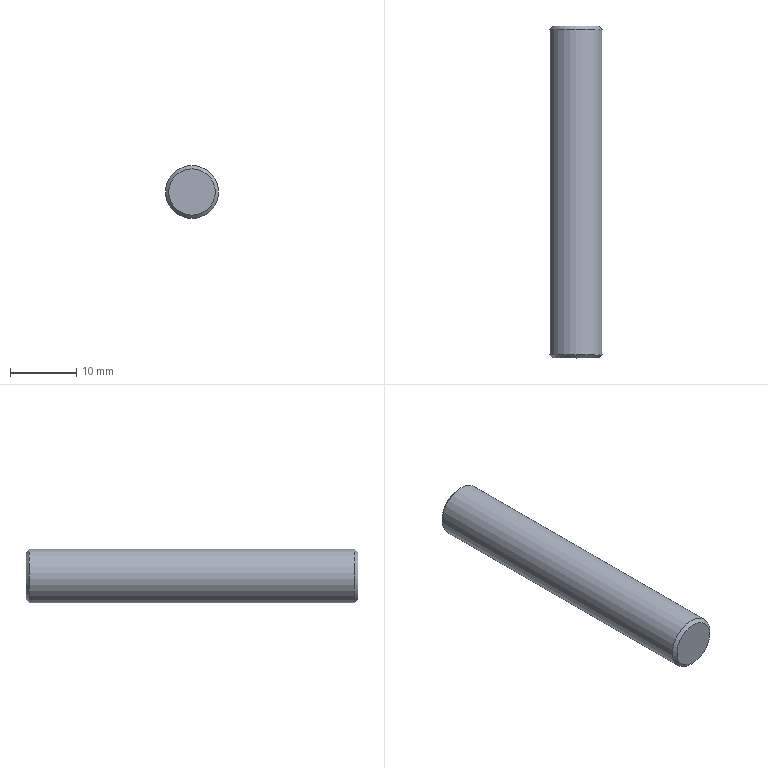Part | STEP file | 车灯-后视镜_id50_x_t | 1 solid | 5 faces | box 8 x 50 x 8 mm | volume 2507 mm3 | plane 2 | cone 2 | cylinder 1 | commonest cylinder face diameters 8 x1
STEP:
#1=CARTESIAN_POINT('',(98.5,-260.,-359.));
#2=VERTEX_POINT('',#1);
#3=CARTESIAN_POINT('',(98.5,-260.,-355.5));
#4=DIRECTION('',(0.,-1.,0.));
#5=DIRECTION('',(0.,0.,-1.));
#6=AXIS2_PLACEMENT_3D('',#3,#4,#5);
#7=CIRCLE('',#6,3.5);
#8=EDGE_CURVE('',#2,#2,#7,.T.);
#9=ORIENTED_EDGE('',*,*,#8,.F.);
#10=EDGE_LOOP('',(#9));
#11=FACE_OUTER_BOUND('',#10,.T.);
#12=CARTESIAN_POINT('',(98.5,-260.,-355.5));
#13=DIRECTION('',(0.,1.,0.));
#14=DIRECTION('',(0.,0.,1.));
#15=AXIS2_PLACEMENT_3D('',#12,#13,#14);
#16=PLANE('',#15);
#17=ADVANCED_FACE('',(#11),#16,.T.);
#18=CARTESIAN_POINT('',(98.5,-310.,-352.));
#19=VERTEX_POINT('',#18);
#20=CARTESIAN_POINT('',(98.5,-310.,-355.5));
#21=DIRECTION('',(0.,1.,0.));
#22=DIRECTION('',(0.,0.,1.));
#23=AXIS2_PLACEMENT_3D('',#20,#21,#22);
#24=CIRCLE('',#23,3.5);
#25=EDGE_CURVE('',#19,#19,#24,.T.);
#26=ORIENTED_EDGE('',*,*,#25,.F.);
#27=EDGE_LOOP('',(#26));
#28=FACE_OUTER_BOUND('',#27,.T.);
#29=CARTESIAN_POINT('',(98.5,-310.,-355.5));
#30=DIRECTION('',(0.,-1.,0.));
#31=DIRECTION('',(0.,0.,-1.));
#32=AXIS2_PLACEMENT_3D('',#29,#30,#31);
#33=PLANE('',#32);
#34=ADVANCED_FACE('',(#28),#33,.T.);
#35=CARTESIAN_POINT('',(98.5,-309.5,-351.5));
#36=VERTEX_POINT('',#35);
#37=CARTESIAN_POINT('',(98.5,-309.5,-355.5));
#38=DIRECTION('',(0.,-1.,0.));
#39=DIRECTION('',(0.,0.,1.));
#40=AXIS2_PLACEMENT_3D('',#37,#38,#39);
#41=CIRCLE('',#40,4.);
#42=EDGE_CURVE('',#36,#36,#41,.T.);
#43=ORIENTED_EDGE('',*,*,#42,.F.);
#44=EDGE_LOOP('',(#43));
#45=FACE_BOUND('',#44,.T.);
#46=CARTESIAN_POINT('',(98.5,-260.5,-359.5));
#47=VERTEX_POINT('',#46);
#48=CARTESIAN_POINT('',(98.5,-260.5,-355.5));
#49=DIRECTION('',(0.,1.,0.));
#50=DIRECTION('',(0.,0.,-1.));
#51=AXIS2_PLACEMENT_3D('',#48,#49,#50);
#52=CIRCLE('',#51,4.);
#53=EDGE_CURVE('',#47,#47,#52,.T.);
#54=ORIENTED_EDGE('',*,*,#53,.F.);
#55=EDGE_LOOP('',(#54));
#56=FACE_BOUND('',#55,.T.);
#57=CARTESIAN_POINT('',(98.5,-310.,-355.5));
#58=DIRECTION('',(0.,1.,0.));
#59=DIRECTION('',(0.,0.,1.));
#60=AXIS2_PLACEMENT_3D('',#57,#58,#59);
#61=CYLINDRICAL_SURFACE('',#60,4.);
#62=ADVANCED_FACE('',(#45,#56),#61,.T.);
#63=ORIENTED_EDGE('',*,*,#25,.T.);
#64=EDGE_LOOP('',(#63));
#65=FACE_BOUND('',#64,.T.);
#66=ORIENTED_EDGE('',*,*,#42,.T.);
#67=EDGE_LOOP('',(#66));
#68=FACE_BOUND('',#67,.T.);
#69=CARTESIAN_POINT('',(98.5,-309.5,-355.5));
#70=DIRECTION('',(0.,1.,0.));
#71=DIRECTION('',(0.,0.,-1.));
#72=AXIS2_PLACEMENT_3D('',#69,#70,#71);
#73=CONICAL_SURFACE('',#72,4.,45.);
#74=ADVANCED_FACE('',(#65,#68),#73,.T.);
#75=ORIENTED_EDGE('',*,*,#8,.T.);
#76=EDGE_LOOP('',(#75));
#77=FACE_BOUND('',#76,.T.);
#78=ORIENTED_EDGE('',*,*,#53,.T.);
#79=EDGE_LOOP('',(#78));
#80=FACE_BOUND('',#79,.T.);
#81=CARTESIAN_POINT('',(98.5,-260.5,-355.5));
#82=DIRECTION('',(0.,-1.,0.));
#83=DIRECTION('',(0.,0.,1.));
#84=AXIS2_PLACEMENT_3D('',#81,#82,#83);
#85=CONICAL_SURFACE('',#84,4.,45.);
#86=ADVANCED_FACE('',(#77,#80),#85,.T.);
#87=CLOSED_SHELL('',(#17,#34,#62,#74,#86));
#88=MANIFOLD_SOLID_BREP('',#87);
#89=(LENGTH_UNIT()NAMED_UNIT(*)SI_UNIT(.MILLI.,.METRE.));
#90=UNCERTAINTY_MEASURE_WITH_UNIT(LENGTH_MEASURE(0.00002),#89,'','');
#91=(NAMED_UNIT(*)PLANE_ANGLE_UNIT()SI_UNIT($,.RADIAN.));
#92=PLANE_ANGLE_MEASURE_WITH_UNIT(PLANE_ANGLE_MEASURE(0.01745),#91);
#93=DIMENSIONAL_EXPONENTS(0.,0.,0.,0.,0.,0.,0.);
#94=(CONVERSION_BASED_UNIT('DEGREE',#92)NAMED_UNIT(#93)PLANE_ANGLE_UNIT());
#95=(NAMED_UNIT(*)SI_UNIT($,.STERADIAN.)SOLID_ANGLE_UNIT());
#96=(GEOMETRIC_REPRESENTATION_CONTEXT(3)GLOBAL_UNCERTAINTY_ASSIGNED_CONTEXT((#90))GLOBAL_UNIT_ASSIGNED_CONTEXT((#89,#94,#95))REPRESENTATION_CONTEXT('',''));
#97=ADVANCED_BREP_SHAPE_REPRESENTATION('',(#88),#96);